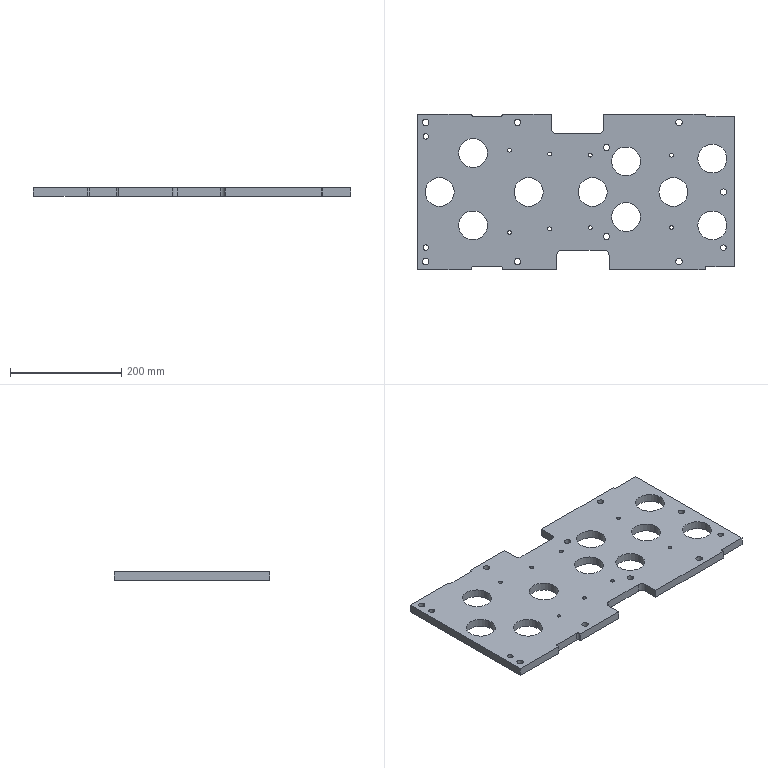Part | NX | features UB-4 2 | 1 solid | 74 faces | box 570 x 280 x 15 mm | volume 1939590 mm3 | cylinder 40 | plane 26 | cone 8 | commonest cylinder face diameters 52.004 x10 11.507 x9 6 x6 6.806 x6 18 x4 10 x3